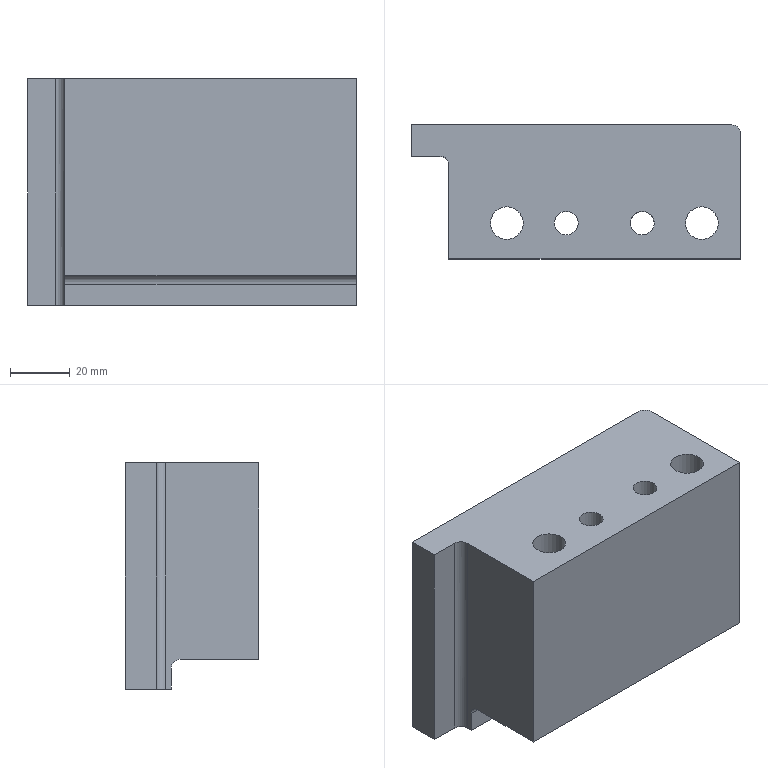Part | NX | features solid 2 | 1 solid | 25 faces | box 110.531 x 45 x 76 mm | volume 284974 mm3 | plane 14 | cylinder 11 | commonest cylinder face diameters 6 x3 8 x2 10.505 x2 11 x2 17 x2
STEP:
#1=CARTESIAN_POINT('',(699.977,-158.1,-43.001));
#2=VERTEX_POINT('',#1);
#3=CARTESIAN_POINT('',(699.977,-147.619,-43.001));
#4=VERTEX_POINT('',#3);
#5=CARTESIAN_POINT('',(699.977,-110.331,-43.001));
#6=DIRECTION('',(0.,-1.,-0.000000517));
#7=VECTOR('',#6,1000.);
#8=LINE('',#5,#7);
#9=EDGE_CURVE('',#2,#4,#8,.F.);
#10=ORIENTED_EDGE('',*,*,#9,.F.);
#11=CARTESIAN_POINT('',(699.977,-158.1,32.999));
#12=VERTEX_POINT('',#11);
#13=CARTESIAN_POINT('',(699.977,-158.101,-70.8));
#14=DIRECTION('',(0.000000053,0.000003911,1.));
#15=VECTOR('',#14,1000.);
#16=LINE('',#13,#15);
#17=EDGE_CURVE('',#12,#2,#16,.F.);
#18=ORIENTED_EDGE('',*,*,#17,.F.);
#19=CARTESIAN_POINT('',(699.977,-147.619,32.999));
#20=VERTEX_POINT('',#19);
#21=CARTESIAN_POINT('',(699.977,-187.619,32.999));
#22=DIRECTION('',(0.,1.,0.000000517));
#23=VECTOR('',#22,1000.);
#24=LINE('',#21,#23);
#25=EDGE_CURVE('',#20,#12,#24,.F.);
#26=ORIENTED_EDGE('',*,*,#25,.F.);
#27=CARTESIAN_POINT('',(699.977,-147.619,56.368));
#28=DIRECTION('',(0.000000053,-0.000000517,1.));
#29=VECTOR('',#28,1000.);
#30=LINE('',#27,#29);
#31=EDGE_CURVE('',#20,#4,#30,.F.);
#32=ORIENTED_EDGE('',*,*,#31,.T.);
#33=EDGE_LOOP('',(#10,#18,#26,#32));
#34=FACE_BOUND('',#33,.T.);
#35=CARTESIAN_POINT('',(699.977,-147.619,-43.001));
#36=DIRECTION('',(1.,0.,-0.000000053));
#37=DIRECTION('',(0.000000053,0.,1.));
#38=AXIS2_PLACEMENT_3D('',#35,#36,#37);
#39=PLANE('',#38);
#40=ADVANCED_FACE('',(#34),#39,.F.);
#41=CARTESIAN_POINT('',(807.509,-147.619,-43.001));
#42=VERTEX_POINT('',#41);
#43=CARTESIAN_POINT('',(574.977,-147.619,-43.001));
#44=DIRECTION('',(1.,0.,-0.000000053));
#45=VECTOR('',#44,1000.);
#46=LINE('',#43,#45);
#47=EDGE_CURVE('',#4,#42,#46,.T.);
#48=ORIENTED_EDGE('',*,*,#47,.T.);
#49=CARTESIAN_POINT('',(810.509,-150.619,-43.001));
#50=VERTEX_POINT('',#49);
#51=CARTESIAN_POINT('',(807.509,-150.619,-43.001));
#52=DIRECTION('',(-0.000000053,0.000000517,-1.));
#53=DIRECTION('',(0.,-1.,-0.000000517));
#54=AXIS2_PLACEMENT_3D('',#51,#52,#53);
#55=CIRCLE('',#54,3.);
#56=EDGE_CURVE('',#50,#42,#55,.F.);
#57=ORIENTED_EDGE('',*,*,#56,.F.);
#58=CARTESIAN_POINT('',(810.509,-163.1,-43.001));
#59=VERTEX_POINT('',#58);
#60=CARTESIAN_POINT('',(810.509,-177.619,-43.001));
#61=DIRECTION('',(0.,1.,0.000000517));
#62=VECTOR('',#61,1000.);
#63=LINE('',#60,#62);
#64=EDGE_CURVE('',#59,#50,#63,.T.);
#65=ORIENTED_EDGE('',*,*,#64,.F.);
#66=CARTESIAN_POINT('',(712.498,-163.1,-43.001));
#67=VERTEX_POINT('',#66);
#68=CARTESIAN_POINT('',(574.977,-163.1,-43.001));
#69=DIRECTION('',(-1.,0.,0.000000053));
#70=VECTOR('',#69,1000.);
#71=LINE('',#68,#70);
#72=EDGE_CURVE('',#59,#67,#71,.T.);
#73=ORIENTED_EDGE('',*,*,#72,.T.);
#74=CARTESIAN_POINT('',(712.498,-161.1,-43.001));
#75=VERTEX_POINT('',#74);
#76=CARTESIAN_POINT('',(712.498,-110.331,-43.001));
#77=DIRECTION('',(0.,1.,0.000000517));
#78=VECTOR('',#77,1000.);
#79=LINE('',#76,#78);
#80=EDGE_CURVE('',#67,#75,#79,.T.);
#81=ORIENTED_EDGE('',*,*,#80,.T.);
#82=CARTESIAN_POINT('',(709.498,-158.1,-43.001));
#83=VERTEX_POINT('',#82);
#84=CARTESIAN_POINT('',(709.498,-161.1,-43.001));
#85=DIRECTION('',(-0.000000053,0.000000517,-1.));
#86=DIRECTION('',(-0.01202,0.9999,0.000000518));
#87=AXIS2_PLACEMENT_3D('',#84,#85,#86);
#88=ELLIPSE('',#87,3.,3.);
#89=EDGE_CURVE('',#75,#83,#88,.F.);
#90=ORIENTED_EDGE('',*,*,#89,.T.);
#91=CARTESIAN_POINT('',(574.977,-158.1,-43.001));
#92=DIRECTION('',(1.,0.,-0.000000053));
#93=VECTOR('',#92,1000.);
#94=LINE('',#91,#93);
#95=EDGE_CURVE('',#83,#2,#94,.F.);
#96=ORIENTED_EDGE('',*,*,#95,.T.);
#97=ORIENTED_EDGE('',*,*,#9,.T.);
#98=EDGE_LOOP('',(#48,#57,#65,#73,#81,#90,#96,#97));
#99=FACE_BOUND('',#98,.T.);
#100=CARTESIAN_POINT('',(574.977,-110.331,-43.001));
#101=DIRECTION('',(-0.000000053,0.000000517,-1.));
#102=DIRECTION('',(1.,0.,-0.000000053));
#103=AXIS2_PLACEMENT_3D('',#100,#101,#102);
#104=PLANE('',#103);
#105=ADVANCED_FACE('',(#99),#104,.T.);
#106=CARTESIAN_POINT('',(807.509,-147.619,32.999));
#107=VERTEX_POINT('',#106);
#108=CARTESIAN_POINT('',(699.977,-147.619,32.999));
#109=DIRECTION('',(-1.,0.,0.000000053));
#110=VECTOR('',#109,1000.);
#111=LINE('',#108,#110);
#112=EDGE_CURVE('',#20,#107,#111,.F.);
#113=ORIENTED_EDGE('',*,*,#112,.T.);
#114=CARTESIAN_POINT('',(807.509,-147.619,56.368));
#115=DIRECTION('',(-0.000000053,0.000000517,-1.));
#116=VECTOR('',#115,1000.);
#117=LINE('',#114,#116);
#118=EDGE_CURVE('',#42,#107,#117,.F.);
#119=ORIENTED_EDGE('',*,*,#118,.F.);
#120=ORIENTED_EDGE('',*,*,#47,.F.);
#121=ORIENTED_EDGE('',*,*,#31,.F.);
#122=EDGE_LOOP('',(#113,#119,#120,#121));
#123=FACE_BOUND('',#122,.T.);
#124=CARTESIAN_POINT('',(583.446,-147.619,56.368));
#125=DIRECTION('',(0.,-1.,-0.000000517));
#126=DIRECTION('',(-0.000000053,0.000000517,-1.));
#127=AXIS2_PLACEMENT_3D('',#124,#125,#126);
#128=PLANE('',#127);
#129=ADVANCED_FACE('',(#123),#128,.F.);
#130=ORIENTED_EDGE('',*,*,#95,.F.);
#131=CARTESIAN_POINT('',(709.498,-158.1,32.999));
#132=VERTEX_POINT('',#131);
#133=CARTESIAN_POINT('',(709.498,-158.1,32.999));
#134=DIRECTION('',(0.,-0.000003911,-1.));
#135=VECTOR('',#134,1000.);
#136=LINE('',#133,#135);
#137=EDGE_CURVE('',#83,#132,#136,.F.);
#138=ORIENTED_EDGE('',*,*,#137,.T.);
#139=CARTESIAN_POINT('',(699.977,-158.1,32.999));
#140=DIRECTION('',(-1.,0.,0.000000053));
#141=VECTOR('',#140,1000.);
#142=LINE('',#139,#141);
#143=EDGE_CURVE('',#132,#12,#142,.T.);
#144=ORIENTED_EDGE('',*,*,#143,.T.);
#145=ORIENTED_EDGE('',*,*,#17,.T.);
#146=EDGE_LOOP('',(#130,#138,#144,#145));
#147=FACE_BOUND('',#146,.T.);
#148=CARTESIAN_POINT('',(704.737,-158.1,-5.001));
#149=DIRECTION('',(0.,-1.,0.000003911));
#150=DIRECTION('',(0.,-0.000003911,-1.));
#151=AXIS2_PLACEMENT_3D('',#148,#149,#150);
#152=PLANE('',#151);
#153=ADVANCED_FACE('',(#147),#152,.T.);
#154=ORIENTED_EDGE('',*,*,#143,.F.);
#155=CARTESIAN_POINT('',(712.498,-161.1,32.999));
#156=VERTEX_POINT('',#155);
#157=CARTESIAN_POINT('',(709.498,-161.1,32.999));
#158=DIRECTION('',(0.000000053,-0.000000517,1.));
#159=DIRECTION('',(-0.01202,0.9999,0.000000518));
#160=AXIS2_PLACEMENT_3D('',#157,#158,#159);
#161=ELLIPSE('',#160,3.,3.);
#162=EDGE_CURVE('',#132,#156,#161,.F.);
#163=ORIENTED_EDGE('',*,*,#162,.T.);
#164=CARTESIAN_POINT('',(712.498,-192.619,32.999));
#165=VERTEX_POINT('',#164);
#166=CARTESIAN_POINT('',(712.498,-187.619,32.999));
#167=DIRECTION('',(0.,-1.,-0.000000517));
#168=VECTOR('',#167,1000.);
#169=LINE('',#166,#168);
#170=EDGE_CURVE('',#165,#156,#169,.F.);
#171=ORIENTED_EDGE('',*,*,#170,.F.);
#172=CARTESIAN_POINT('',(810.509,-192.619,32.999));
#173=VERTEX_POINT('',#172);
#174=CARTESIAN_POINT('',(699.977,-192.619,32.999));
#175=DIRECTION('',(-1.,0.,0.000000053));
#176=VECTOR('',#175,1000.);
#177=LINE('',#174,#176);
#178=EDGE_CURVE('',#165,#173,#177,.F.);
#179=ORIENTED_EDGE('',*,*,#178,.T.);
#180=CARTESIAN_POINT('',(810.509,-150.619,32.999));
#181=VERTEX_POINT('',#180);
#182=CARTESIAN_POINT('',(810.509,-177.619,32.999));
#183=DIRECTION('',(0.,-1.,-0.000000517));
#184=VECTOR('',#183,1000.);
#185=LINE('',#182,#184);
#186=EDGE_CURVE('',#173,#181,#185,.F.);
#187=ORIENTED_EDGE('',*,*,#186,.T.);
#188=CARTESIAN_POINT('',(807.509,-150.619,32.999));
#189=DIRECTION('',(0.000000053,-0.000000517,1.));
#190=DIRECTION('',(0.,1.,0.000000517));
#191=AXIS2_PLACEMENT_3D('',#188,#189,#190);
#192=CIRCLE('',#191,3.);
#193=EDGE_CURVE('',#181,#107,#192,.T.);
#194=ORIENTED_EDGE('',*,*,#193,.T.);
#195=ORIENTED_EDGE('',*,*,#112,.F.);
#196=ORIENTED_EDGE('',*,*,#25,.T.);
#197=EDGE_LOOP('',(#154,#163,#171,#179,#187,#194,#195,#196));
#198=FACE_BOUND('',#197,.T.);
#199=CARTESIAN_POINT('',(797.509,-186.119,32.999));
#200=VERTEX_POINT('',#199);
#201=CARTESIAN_POINT('',(797.509,-180.619,32.999));
#202=DIRECTION('',(0.000000053,-0.000000517,1.));
#203=DIRECTION('',(0.,-1.,-0.000000517));
#204=AXIS2_PLACEMENT_3D('',#201,#202,#203);
#205=CIRCLE('',#204,5.5);
#206=EDGE_CURVE('',#200,#200,#205,.F.);
#207=ORIENTED_EDGE('',*,*,#206,.T.);
#208=EDGE_LOOP('',(#207));
#209=FACE_BOUND('',#208,.T.);
#210=CARTESIAN_POINT('',(731.977,-186.119,32.999));
#211=VERTEX_POINT('',#210);
#212=CARTESIAN_POINT('',(731.977,-180.619,32.999));
#213=DIRECTION('',(0.000000053,-0.000000517,1.));
#214=DIRECTION('',(0.,-1.,-0.000000517));
#215=AXIS2_PLACEMENT_3D('',#212,#213,#214);
#216=CIRCLE('',#215,5.5);
#217=EDGE_CURVE('',#211,#211,#216,.F.);
#218=ORIENTED_EDGE('',*,*,#217,.T.);
#219=EDGE_LOOP('',(#218));
#220=FACE_BOUND('',#219,.T.);
#221=CARTESIAN_POINT('',(777.509,-184.619,32.999));
#222=VERTEX_POINT('',#221);
#223=CARTESIAN_POINT('',(777.509,-180.619,32.999));
#224=DIRECTION('',(-0.000000053,0.000000517,-1.));
#225=DIRECTION('',(0.,-1.,-0.000000517));
#226=AXIS2_PLACEMENT_3D('',#223,#224,#225);
#227=CIRCLE('',#226,4.);
#228=EDGE_CURVE('',#222,#222,#227,.T.);
#229=ORIENTED_EDGE('',*,*,#228,.T.);
#230=EDGE_LOOP('',(#229));
#231=FACE_BOUND('',#230,.T.);
#232=CARTESIAN_POINT('',(751.977,-184.619,32.999));
#233=VERTEX_POINT('',#232);
#234=CARTESIAN_POINT('',(751.977,-180.619,32.999));
#235=DIRECTION('',(-0.000000053,0.000000517,-1.));
#236=DIRECTION('',(0.,-1.,-0.000000517));
#237=AXIS2_PLACEMENT_3D('',#234,#235,#236);
#238=CIRCLE('',#237,4.);
#239=EDGE_CURVE('',#233,#233,#238,.T.);
#240=ORIENTED_EDGE('',*,*,#239,.T.);
#241=EDGE_LOOP('',(#240));
#242=FACE_BOUND('',#241,.T.);
#243=CARTESIAN_POINT('',(699.977,-187.619,32.999));
#244=DIRECTION('',(0.000000053,-0.000000517,1.));
#245=DIRECTION('',(1.,0.,-0.000000053));
#246=AXIS2_PLACEMENT_3D('',#243,#244,#245);
#247=PLANE('',#246);
#248=ADVANCED_FACE('',(#198,#209,#220,#231,#242),#247,.T.);
#249=CARTESIAN_POINT('',(810.509,-163.1,-36.001));
#250=VERTEX_POINT('',#249);
#251=CARTESIAN_POINT('',(810.509,-163.1,-5.001));
#252=DIRECTION('',(0.000000053,0.000003911,1.));
#253=VECTOR('',#252,1000.);
#254=LINE('',#251,#253);
#255=EDGE_CURVE('',#59,#250,#254,.T.);
#256=ORIENTED_EDGE('',*,*,#255,.T.);
#257=CARTESIAN_POINT('',(712.498,-163.1,-36.001));
#258=VERTEX_POINT('',#257);
#259=CARTESIAN_POINT('',(712.498,-163.1,-36.001));
#260=DIRECTION('',(1.,0.,-0.000000053));
#261=VECTOR('',#260,1000.);
#262=LINE('',#259,#261);
#263=EDGE_CURVE('',#250,#258,#262,.F.);
#264=ORIENTED_EDGE('',*,*,#263,.T.);
#265=CARTESIAN_POINT('',(712.498,-163.1,49.2));
#266=DIRECTION('',(0.,0.000003911,1.));
#267=VECTOR('',#266,1000.);
#268=LINE('',#265,#267);
#269=EDGE_CURVE('',#67,#258,#268,.T.);
#270=ORIENTED_EDGE('',*,*,#269,.F.);
#271=ORIENTED_EDGE('',*,*,#72,.F.);
#272=EDGE_LOOP('',(#256,#264,#270,#271));
#273=FACE_BOUND('',#272,.T.);
#274=CARTESIAN_POINT('',(704.737,-163.1,-5.001));
#275=DIRECTION('',(0.,-1.,0.000003911));
#276=DIRECTION('',(0.,-0.000003911,-1.));
#277=AXIS2_PLACEMENT_3D('',#274,#275,#276);
#278=PLANE('',#277);
#279=ADVANCED_FACE('',(#273),#278,.T.);
#280=ORIENTED_EDGE('',*,*,#186,.F.);
#281=CARTESIAN_POINT('',(810.509,-192.619,-33.001));
#282=VERTEX_POINT('',#281);
#283=CARTESIAN_POINT('',(810.509,-192.619,-43.001));
#284=DIRECTION('',(0.000000053,-0.000000517,1.));
#285=VECTOR('',#284,1000.);
#286=LINE('',#283,#285);
#287=EDGE_CURVE('',#173,#282,#286,.F.);
#288=ORIENTED_EDGE('',*,*,#287,.T.);
#289=CARTESIAN_POINT('',(810.509,-166.1,-33.001));
#290=VERTEX_POINT('',#289);
#291=CARTESIAN_POINT('',(810.509,-177.619,-33.001));
#292=DIRECTION('',(0.,1.,0.000000517));
#293=VECTOR('',#292,1000.);
#294=LINE('',#291,#293);
#295=EDGE_CURVE('',#282,#290,#294,.T.);
#296=ORIENTED_EDGE('',*,*,#295,.T.);
#297=CARTESIAN_POINT('',(810.509,-166.1,-36.001));
#298=DIRECTION('',(1.,0.,-0.000000053));
#299=DIRECTION('',(-0.000000053,0.,-1.));
#300=AXIS2_PLACEMENT_3D('',#297,#298,#299);
#301=CIRCLE('',#300,3.);
#302=EDGE_CURVE('',#290,#250,#301,.F.);
#303=ORIENTED_EDGE('',*,*,#302,.T.);
#304=ORIENTED_EDGE('',*,*,#255,.F.);
#305=ORIENTED_EDGE('',*,*,#64,.T.);
#306=CARTESIAN_POINT('',(810.509,-150.619,-43.001));
#307=DIRECTION('',(-0.000000053,0.000000517,-1.));
#308=VECTOR('',#307,1000.);
#309=LINE('',#306,#308);
#310=EDGE_CURVE('',#181,#50,#309,.T.);
#311=ORIENTED_EDGE('',*,*,#310,.F.);
#312=EDGE_LOOP('',(#280,#288,#296,#303,#304,#305,#311));
#313=FACE_BOUND('',#312,.T.);
#314=CARTESIAN_POINT('',(810.509,-177.619,-43.001));
#315=DIRECTION('',(1.,0.,-0.000000053));
#316=DIRECTION('',(0.000000053,-0.000000517,1.));
#317=AXIS2_PLACEMENT_3D('',#314,#315,#316);
#318=PLANE('',#317);
#319=ADVANCED_FACE('',(#313),#318,.T.);
#320=ORIENTED_EDGE('',*,*,#178,.F.);
#321=CARTESIAN_POINT('',(712.498,-192.619,-33.001));
#322=VERTEX_POINT('',#321);
#323=CARTESIAN_POINT('',(712.498,-192.619,-43.001));
#324=DIRECTION('',(0.,0.000000517,-1.));
#325=VECTOR('',#324,1000.);
#326=LINE('',#323,#325);
#327=EDGE_CURVE('',#165,#322,#326,.T.);
#328=ORIENTED_EDGE('',*,*,#327,.T.);
#329=CARTESIAN_POINT('',(574.977,-192.619,-33.001));
#330=DIRECTION('',(-1.,0.,0.000000053));
#331=VECTOR('',#330,1000.);
#332=LINE('',#329,#331);
#333=EDGE_CURVE('',#282,#322,#332,.T.);
#334=ORIENTED_EDGE('',*,*,#333,.F.);
#335=ORIENTED_EDGE('',*,*,#287,.F.);
#336=EDGE_LOOP('',(#320,#328,#334,#335));
#337=FACE_BOUND('',#336,.T.);
#338=CARTESIAN_POINT('',(699.977,-192.619,-43.001));
#339=DIRECTION('',(0.,-1.,-0.000000517));
#340=DIRECTION('',(-0.000000053,0.000000517,-1.));
#341=AXIS2_PLACEMENT_3D('',#338,#339,#340);
#342=PLANE('',#341);
#343=ADVANCED_FACE('',(#337),#342,.T.);
#344=ORIENTED_EDGE('',*,*,#170,.T.);
#345=CARTESIAN_POINT('',(712.498,-161.1,-43.001));
#346=DIRECTION('',(0.,-0.000003911,-1.));
#347=VECTOR('',#346,1000.);
#348=LINE('',#345,#347);
#349=EDGE_CURVE('',#156,#75,#348,.T.);
#350=ORIENTED_EDGE('',*,*,#349,.T.);
#351=ORIENTED_EDGE('',*,*,#80,.F.);
#352=ORIENTED_EDGE('',*,*,#269,.T.);
#353=CARTESIAN_POINT('',(712.498,-166.1,-33.001));
#354=VERTEX_POINT('',#353);
#355=CARTESIAN_POINT('',(712.498,-166.1,-36.001));
#356=DIRECTION('',(-1.,0.,0.));
#357=DIRECTION('',(0.,-1.,0.));
#358=AXIS2_PLACEMENT_3D('',#355,#356,#357);
#359=CIRCLE('',#358,3.);
#360=EDGE_CURVE('',#258,#354,#359,.F.);
#361=ORIENTED_EDGE('',*,*,#360,.T.);
#362=CARTESIAN_POINT('',(712.498,-110.331,-33.001));
#363=DIRECTION('',(0.,1.,0.000000517));
#364=VECTOR('',#363,1000.);
#365=LINE('',#362,#364);
#366=EDGE_CURVE('',#322,#354,#365,.T.);
#367=ORIENTED_EDGE('',*,*,#366,.F.);
#368=ORIENTED_EDGE('',*,*,#327,.F.);
#369=EDGE_LOOP('',(#344,#350,#351,#352,#361,#367,#368));
#370=FACE_BOUND('',#369,.T.);
#371=CARTESIAN_POINT('',(712.498,-177.1,49.2));
#372=DIRECTION('',(-1.,0.,0.));
#373=DIRECTION('',(0.,-1.,0.000003329));
#374=AXIS2_PLACEMENT_3D('',#371,#372,#373);
#375=PLANE('',#374);
#376=ADVANCED_FACE('',(#370),#375,.T.);
#377=ORIENTED_EDGE('',*,*,#366,.T.);
#378=CARTESIAN_POINT('',(810.509,-166.1,-33.001));
#379=DIRECTION('',(1.,0.,-0.000000053));
#380=VECTOR('',#379,1000.);
#381=LINE('',#378,#380);
#382=EDGE_CURVE('',#354,#290,#381,.T.);
#383=ORIENTED_EDGE('',*,*,#382,.T.);
#384=ORIENTED_EDGE('',*,*,#295,.F.);
#385=ORIENTED_EDGE('',*,*,#333,.T.);
#386=EDGE_LOOP('',(#377,#383,#384,#385));
#387=FACE_BOUND('',#386,.T.);
#388=CARTESIAN_POINT('',(731.977,-172.119,-33.001));
#389=VERTEX_POINT('',#388);
#390=CARTESIAN_POINT('',(731.977,-180.619,-33.001));
#391=DIRECTION('',(-0.000000053,0.000000517,-1.));
#392=DIRECTION('',(0.,1.,0.000000517));
#393=AXIS2_PLACEMENT_3D('',#390,#391,#392);
#394=CIRCLE('',#393,8.5);
#395=EDGE_CURVE('',#389,#389,#394,.T.);
#396=ORIENTED_EDGE('',*,*,#395,.F.);
#397=EDGE_LOOP('',(#396));
#398=FACE_BOUND('',#397,.T.);
#399=CARTESIAN_POINT('',(751.977,-175.366,-33.001));
#400=VERTEX_POINT('',#399);
#401=CARTESIAN_POINT('',(753.045,-175.439,-33.001));
#402=CARTESIAN_POINT('',(752.012,-175.332,-33.001));
#403=CARTESIAN_POINT('',(750.981,-175.429,-33.001));
#404=CARTESIAN_POINT('',(750.004,-175.714,-33.001));
#405=CARTESIAN_POINT('',(749.086,-176.193,-33.001));
#406=CARTESIAN_POINT('',(748.278,-176.842,-33.001));
#407=CARTESIAN_POINT('',(747.613,-177.636,-33.001));
#408=CARTESIAN_POINT('',(747.115,-178.545,-33.001));
#409=CARTESIAN_POINT('',(746.803,-179.533,-33.001));
#410=CARTESIAN_POINT('',(746.691,-180.564,-33.001));
#411=CARTESIAN_POINT('',(746.782,-181.596,-33.001));
#412=CARTESIAN_POINT('',(747.073,-182.591,-33.001));
#413=CARTESIAN_POINT('',(747.552,-183.51,-33.001));
#414=CARTESIAN_POINT('',(748.201,-184.318,-33.001));
#415=CARTESIAN_POINT('',(748.995,-184.983,-33.001));
#416=CARTESIAN_POINT('',(749.904,-185.481,-33.001));
#417=CARTESIAN_POINT('',(750.892,-185.792,-33.001));
#418=CARTESIAN_POINT('',(751.922,-185.905,-33.001));
#419=CARTESIAN_POINT('',(752.955,-185.814,-33.001));
#420=CARTESIAN_POINT('',(753.95,-185.523,-33.001));
#421=CARTESIAN_POINT('',(754.868,-185.044,-33.001));
#422=CARTESIAN_POINT('',(755.676,-184.395,-33.001));
#423=CARTESIAN_POINT('',(756.342,-183.601,-33.001));
#424=CARTESIAN_POINT('',(756.84,-182.692,-33.001));
#425=CARTESIAN_POINT('',(757.151,-181.704,-33.001));
#426=CARTESIAN_POINT('',(757.263,-180.673,-33.001));
#427=CARTESIAN_POINT('',(757.172,-179.641,-33.001));
#428=CARTESIAN_POINT('',(756.882,-178.646,-33.001));
#429=CARTESIAN_POINT('',(756.403,-177.727,-33.001));
#430=CARTESIAN_POINT('',(755.754,-176.919,-33.001));
#431=CARTESIAN_POINT('',(754.96,-176.254,-33.001));
#432=CARTESIAN_POINT('',(754.051,-175.756,-33.001));
#433=CARTESIAN_POINT('',(753.045,-175.439,-33.001));
#434=CARTESIAN_POINT('',(752.012,-175.332,-33.001));
#435=CARTESIAN_POINT('',(750.981,-175.429,-33.001));
#436=B_SPLINE_CURVE_WITH_KNOTS('',3,(#401,#402,#403,#404,#405,#406,#407,#408,#409,#410,#411,#412,#413,#414,#415,#416,#417,#418,#419,#420,#421,#422,#423,#424,#425,#426,#427,#428,#429,#430,#431,#432,#433,#434,#435),.UNSPECIFIED.,.T.,.F.,(1,1,1,1,1,1,1,1,1,1,1,1,1,1,1,1,1,1,1,1,1,1,1,1,1,1,1,1,1,1,1,1,1,1,1,1,1,1,1),(-0.09539,-0.06414,-0.03289,0.,0.02969,0.06086,0.09211,0.1234,0.1546,0.1859,0.2171,0.2484,0.2796,0.3109,0.3421,0.3734,0.4046,0.4359,0.4671,0.4984,0.5296,0.5609,0.5921,0.6234,0.6546,0.6859,0.7171,0.7484,0.7796,0.8109,0.8421,0.8734,0.9046,0.9359,0.9671,1.,1.03,1.061,1.092),.UNSPECIFIED.);
#437=EDGE_CURVE('',#400,#400,#436,.F.);
#438=ORIENTED_EDGE('',*,*,#437,.F.);
#439=EDGE_LOOP('',(#438));
#440=FACE_BOUND('',#439,.T.);
#441=CARTESIAN_POINT('',(777.509,-175.366,-33.001));
#442=VERTEX_POINT('',#441);
#443=CARTESIAN_POINT('',(776.441,-175.439,-33.001));
#444=CARTESIAN_POINT('',(777.473,-175.332,-33.001));
#445=CARTESIAN_POINT('',(778.504,-175.429,-33.001));
#446=CARTESIAN_POINT('',(779.482,-175.714,-33.001));
#447=CARTESIAN_POINT('',(780.4,-176.193,-33.001));
#448=CARTESIAN_POINT('',(781.208,-176.842,-33.001));
#449=CARTESIAN_POINT('',(781.873,-177.636,-33.001));
#450=CARTESIAN_POINT('',(782.371,-178.545,-33.001));
#451=CARTESIAN_POINT('',(782.682,-179.533,-33.001));
#452=CARTESIAN_POINT('',(782.795,-180.564,-33.001));
#453=CARTESIAN_POINT('',(782.704,-181.596,-33.001));
#454=CARTESIAN_POINT('',(782.413,-182.591,-33.001));
#455=CARTESIAN_POINT('',(781.934,-183.51,-33.001));
#456=CARTESIAN_POINT('',(781.285,-184.318,-33.001));
#457=CARTESIAN_POINT('',(780.491,-184.983,-33.001));
#458=CARTESIAN_POINT('',(779.582,-185.481,-33.001));
#459=CARTESIAN_POINT('',(778.594,-185.792,-33.001));
#460=CARTESIAN_POINT('',(777.563,-185.905,-33.001));
#461=CARTESIAN_POINT('',(776.531,-185.814,-33.001));
#462=CARTESIAN_POINT('',(775.536,-185.523,-33.001));
#463=CARTESIAN_POINT('',(774.617,-185.044,-33.001));
#464=CARTESIAN_POINT('',(773.81,-184.395,-33.001));
#465=CARTESIAN_POINT('',(773.144,-183.601,-33.001));
#466=CARTESIAN_POINT('',(772.646,-182.692,-33.001));
#467=CARTESIAN_POINT('',(772.335,-181.704,-33.001));
#468=CARTESIAN_POINT('',(772.222,-180.673,-33.001));
#469=CARTESIAN_POINT('',(772.313,-179.641,-33.001));
#470=CARTESIAN_POINT('',(772.604,-178.646,-33.001));
#471=CARTESIAN_POINT('',(773.083,-177.727,-33.001));
#472=CARTESIAN_POINT('',(773.732,-176.919,-33.001));
#473=CARTESIAN_POINT('',(774.526,-176.254,-33.001));
#474=CARTESIAN_POINT('',(775.435,-175.756,-33.001));
#475=CARTESIAN_POINT('',(776.441,-175.439,-33.001));
#476=CARTESIAN_POINT('',(777.473,-175.332,-33.001));
#477=CARTESIAN_POINT('',(778.504,-175.429,-33.001));
#478=B_SPLINE_CURVE_WITH_KNOTS('',3,(#443,#444,#445,#446,#447,#448,#449,#450,#451,#452,#453,#454,#455,#456,#457,#458,#459,#460,#461,#462,#463,#464,#465,#466,#467,#468,#469,#470,#471,#472,#473,#474,#475,#476,#477),.UNSPECIFIED.,.T.,.F.,(1,1,1,1,1,1,1,1,1,1,1,1,1,1,1,1,1,1,1,1,1,1,1,1,1,1,1,1,1,1,1,1,1,1,1,1,1,1,1),(-0.09539,-0.06414,-0.03289,0.,0.02969,0.06086,0.09211,0.1234,0.1546,0.1859,0.2171,0.2484,0.2796,0.3109,0.3421,0.3734,0.4046,0.4359,0.4671,0.4984,0.5296,0.5609,0.5921,0.6234,0.6546,0.6859,0.7171,0.7484,0.7796,0.8109,0.8421,0.8734,0.9046,0.9359,0.9671,1.,1.03,1.061,1.092),.UNSPECIFIED.);
#479=EDGE_CURVE('',#442,#442,#478,.T.);
#480=ORIENTED_EDGE('',*,*,#479,.F.);
#481=EDGE_LOOP('',(#480));
#482=FACE_BOUND('',#481,.T.);
#483=CARTESIAN_POINT('',(797.509,-172.119,-33.001));
#484=VERTEX_POINT('',#483);
#485=CARTESIAN_POINT('',(797.509,-180.619,-33.001));
#486=DIRECTION('',(-0.000000053,0.000000517,-1.));
#487=DIRECTION('',(0.,1.,0.000000517));
#488=AXIS2_PLACEMENT_3D('',#485,#486,#487);
#489=CIRCLE('',#488,8.5);
#490=EDGE_CURVE('',#484,#484,#489,.T.);
#491=ORIENTED_EDGE('',*,*,#490,.F.);
#492=EDGE_LOOP('',(#491));
#493=FACE_BOUND('',#492,.T.);
#494=CARTESIAN_POINT('',(574.977,-110.331,-33.001));
#495=DIRECTION('',(-0.000000053,0.000000517,-1.));
#496=DIRECTION('',(1.,0.,-0.000000053));
#497=AXIS2_PLACEMENT_3D('',#494,#495,#496);
#498=PLANE('',#497);
#499=ADVANCED_FACE('',(#387,#398,#440,#482,#493),#498,.T.);
#500=CARTESIAN_POINT('',(797.509,-175.119,7.999));
#501=VERTEX_POINT('',#500);
#502=CARTESIAN_POINT('',(797.509,-180.619,7.999));
#503=DIRECTION('',(-0.00000016,0.000000517,-1.));
#504=DIRECTION('',(0.,1.,0.000000517));
#505=AXIS2_PLACEMENT_3D('',#502,#503,#504);
#506=CIRCLE('',#505,5.5);
#507=EDGE_CURVE('',#501,#501,#506,.T.);
#508=ORIENTED_EDGE('',*,*,#507,.T.);
#509=EDGE_LOOP('',(#508));
#510=FACE_BOUND('',#509,.T.);
#511=ORIENTED_EDGE('',*,*,#206,.F.);
#512=EDGE_LOOP('',(#511));
#513=FACE_BOUND('',#512,.T.);
#514=CARTESIAN_POINT('',(797.509,-180.619,33.999));
#515=DIRECTION('',(-0.00000016,0.000000517,-1.));
#516=DIRECTION('',(0.,-1.,-0.000000517));
#517=AXIS2_PLACEMENT_3D('',#514,#515,#516);
#518=CYLINDRICAL_SURFACE('',#517,5.5);
#519=ADVANCED_FACE('',(#510,#513),#518,.F.);
#520=ORIENTED_EDGE('',*,*,#490,.T.);
#521=EDGE_LOOP('',(#520));
#522=FACE_BOUND('',#521,.T.);
#523=CARTESIAN_POINT('',(797.509,-172.119,7.999));
#524=VERTEX_POINT('',#523);
#525=CARTESIAN_POINT('',(797.509,-180.619,7.999));
#526=DIRECTION('',(-0.00000016,0.000000517,-1.));
#527=DIRECTION('',(0.,1.,0.000000517));
#528=AXIS2_PLACEMENT_3D('',#525,#526,#527);
#529=CIRCLE('',#528,8.5);
#530=EDGE_CURVE('',#524,#524,#529,.F.);
#531=ORIENTED_EDGE('',*,*,#530,.T.);
#532=EDGE_LOOP('',(#531));
#533=FACE_BOUND('',#532,.T.);
#534=CARTESIAN_POINT('',(797.509,-180.619,7.999));
#535=DIRECTION('',(-0.00000016,0.000000517,-1.));
#536=DIRECTION('',(0.,-1.,-0.000000517));
#537=AXIS2_PLACEMENT_3D('',#534,#535,#536);
#538=CYLINDRICAL_SURFACE('',#537,8.5);
#539=ADVANCED_FACE('',(#522,#533),#538,.F.);
#540=ORIENTED_EDGE('',*,*,#507,.F.);
#541=EDGE_LOOP('',(#540));
#542=FACE_BOUND('',#541,.T.);
#543=ORIENTED_EDGE('',*,*,#530,.F.);
#544=EDGE_LOOP('',(#543));
#545=FACE_BOUND('',#544,.T.);
#546=CARTESIAN_POINT('',(797.509,-180.619,7.999));
#547=DIRECTION('',(-0.00000016,0.000000517,-1.));
#548=DIRECTION('',(0.,-1.,-0.000000517));
#549=AXIS2_PLACEMENT_3D('',#546,#547,#548);
#550=PLANE('',#549);
#551=ADVANCED_FACE('',(#542,#545),#550,.T.);
#552=CARTESIAN_POINT('',(781.509,-180.618,-13.001));
#553=VERTEX_POINT('',#552);
#554=CARTESIAN_POINT('',(777.509,-180.618,-13.001));
#555=DIRECTION('',(-0.000000874,-0.000001551,1.));
#556=DIRECTION('',(1.,0.,0.000000874));
#557=AXIS2_PLACEMENT_3D('',#554,#555,#556);
#558=CIRCLE('',#557,4.);
#559=EDGE_CURVE('',#553,#553,#558,.F.);
#560=ORIENTED_EDGE('',*,*,#559,.T.);
#561=EDGE_LOOP('',(#560));
#562=FACE_BOUND('',#561,.T.);
#563=ORIENTED_EDGE('',*,*,#228,.F.);
#564=EDGE_LOOP('',(#563));
#565=FACE_BOUND('',#564,.T.);
#566=CARTESIAN_POINT('',(777.509,-180.619,33.999));
#567=DIRECTION('',(0.000000874,0.000001551,-1.));
#568=DIRECTION('',(0.,-1.,-0.000001551));
#569=AXIS2_PLACEMENT_3D('',#566,#567,#568);
#570=CYLINDRICAL_SURFACE('',#569,4.);
#571=ADVANCED_FACE('',(#562,#565),#570,.F.);
#572=ORIENTED_EDGE('',*,*,#479,.T.);
#573=EDGE_LOOP('',(#572));
#574=FACE_BOUND('',#573,.T.);
#575=CARTESIAN_POINT('',(782.761,-180.618,-13.001));
#576=VERTEX_POINT('',#575);
#577=CARTESIAN_POINT('',(777.509,-180.618,-13.001));
#578=DIRECTION('',(-0.000000874,-0.000001551,1.));
#579=DIRECTION('',(1.,0.,0.000000874));
#580=AXIS2_PLACEMENT_3D('',#577,#578,#579);
#581=CIRCLE('',#580,5.253);
#582=EDGE_CURVE('',#576,#576,#581,.T.);
#583=ORIENTED_EDGE('',*,*,#582,.T.);
#584=EDGE_LOOP('',(#583));
#585=FACE_BOUND('',#584,.T.);
#586=CARTESIAN_POINT('',(777.509,-180.618,-33.001));
#587=DIRECTION('',(0.000000874,0.000001551,-1.));
#588=DIRECTION('',(0.,-1.,-0.000001551));
#589=AXIS2_PLACEMENT_3D('',#586,#587,#588);
#590=CYLINDRICAL_SURFACE('',#589,5.253);
#591=ADVANCED_FACE('',(#574,#585),#590,.F.);
#592=ORIENTED_EDGE('',*,*,#559,.F.);
#593=EDGE_LOOP('',(#592));
#594=FACE_BOUND('',#593,.T.);
#595=ORIENTED_EDGE('',*,*,#582,.F.);
#596=EDGE_LOOP('',(#595));
#597=FACE_BOUND('',#596,.T.);
#598=CARTESIAN_POINT('',(777.509,-180.618,-13.001));
#599=DIRECTION('',(0.000000874,0.000001551,-1.));
#600=DIRECTION('',(0.,-1.,-0.000001551));
#601=AXIS2_PLACEMENT_3D('',#598,#599,#600);
#602=PLANE('',#601);
#603=ADVANCED_FACE('',(#594,#597),#602,.T.);
#604=CARTESIAN_POINT('',(751.977,-184.619,-13.001));
#605=VERTEX_POINT('',#604);
#606=CARTESIAN_POINT('',(751.977,-180.619,-13.001));
#607=DIRECTION('',(0.000001087,-0.000001551,1.));
#608=DIRECTION('',(0.,-1.,-0.000001551));
#609=AXIS2_PLACEMENT_3D('',#606,#607,#608);
#610=CIRCLE('',#609,4.);
#611=EDGE_CURVE('',#605,#605,#610,.T.);
#612=ORIENTED_EDGE('',*,*,#611,.F.);
#613=EDGE_LOOP('',(#612));
#614=FACE_BOUND('',#613,.T.);
#615=ORIENTED_EDGE('',*,*,#239,.F.);
#616=EDGE_LOOP('',(#615));
#617=FACE_BOUND('',#616,.T.);
#618=CARTESIAN_POINT('',(751.977,-180.619,33.999));
#619=DIRECTION('',(-0.000001087,0.000001551,-1.));
#620=DIRECTION('',(0.,-1.,-0.000001551));
#621=AXIS2_PLACEMENT_3D('',#618,#619,#620);
#622=CYLINDRICAL_SURFACE('',#621,4.);
#623=ADVANCED_FACE('',(#614,#617),#622,.F.);
#624=ORIENTED_EDGE('',*,*,#437,.T.);
#625=EDGE_LOOP('',(#624));
#626=FACE_BOUND('',#625,.T.);
#627=CARTESIAN_POINT('',(746.725,-180.619,-13.001));
#628=VERTEX_POINT('',#627);
#629=CARTESIAN_POINT('',(751.977,-180.619,-13.001));
#630=DIRECTION('',(0.000001087,-0.000001551,1.));
#631=DIRECTION('',(-1.,0.,0.000001087));
#632=AXIS2_PLACEMENT_3D('',#629,#630,#631);
#633=CIRCLE('',#632,5.253);
#634=EDGE_CURVE('',#628,#628,#633,.F.);
#635=ORIENTED_EDGE('',*,*,#634,.F.);
#636=EDGE_LOOP('',(#635));
#637=FACE_BOUND('',#636,.T.);
#638=CARTESIAN_POINT('',(751.977,-180.619,-33.001));
#639=DIRECTION('',(-0.000001087,0.000001551,-1.));
#640=DIRECTION('',(0.,-1.,-0.000001551));
#641=AXIS2_PLACEMENT_3D('',#638,#639,#640);
#642=CYLINDRICAL_SURFACE('',#641,5.253);
#643=ADVANCED_FACE('',(#626,#637),#642,.F.);
#644=ORIENTED_EDGE('',*,*,#611,.T.);
#645=EDGE_LOOP('',(#644));
#646=FACE_BOUND('',#645,.T.);
#647=ORIENTED_EDGE('',*,*,#634,.T.);
#648=EDGE_LOOP('',(#647));
#649=FACE_BOUND('',#648,.T.);
#650=CARTESIAN_POINT('',(751.977,-180.619,-13.001));
#651=DIRECTION('',(-0.000001087,0.000001551,-1.));
#652=DIRECTION('',(0.,-1.,-0.000001551));
#653=AXIS2_PLACEMENT_3D('',#650,#651,#652);
#654=PLANE('',#653);
#655=ADVANCED_FACE('',(#646,#649),#654,.T.);
#656=CARTESIAN_POINT('',(731.977,-175.119,7.999));
#657=VERTEX_POINT('',#656);
#658=CARTESIAN_POINT('',(731.977,-180.619,7.999));
#659=DIRECTION('',(-0.000000053,0.000000517,-1.));
#660=DIRECTION('',(0.,1.,0.000000517));
#661=AXIS2_PLACEMENT_3D('',#658,#659,#660);
#662=CIRCLE('',#661,5.5);
#663=EDGE_CURVE('',#657,#657,#662,.F.);
#664=ORIENTED_EDGE('',*,*,#663,.F.);
#665=EDGE_LOOP('',(#664));
#666=FACE_BOUND('',#665,.T.);
#667=ORIENTED_EDGE('',*,*,#217,.F.);
#668=EDGE_LOOP('',(#667));
#669=FACE_BOUND('',#668,.T.);
#670=CARTESIAN_POINT('',(731.977,-180.619,33.999));
#671=DIRECTION('',(-0.000000053,0.000000517,-1.));
#672=DIRECTION('',(0.,-1.,-0.000000517));
#673=AXIS2_PLACEMENT_3D('',#670,#671,#672);
#674=CYLINDRICAL_SURFACE('',#673,5.5);
#675=ADVANCED_FACE('',(#666,#669),#674,.F.);
#676=ORIENTED_EDGE('',*,*,#395,.T.);
#677=EDGE_LOOP('',(#676));
#678=FACE_BOUND('',#677,.T.);
#679=CARTESIAN_POINT('',(731.977,-172.119,7.999));
#680=VERTEX_POINT('',#679);
#681=CARTESIAN_POINT('',(731.977,-180.619,7.999));
#682=DIRECTION('',(-0.000000053,0.000000517,-1.));
#683=DIRECTION('',(0.,1.,0.000000517));
#684=AXIS2_PLACEMENT_3D('',#681,#682,#683);
#685=CIRCLE('',#684,8.5);
#686=EDGE_CURVE('',#680,#680,#685,.T.);
#687=ORIENTED_EDGE('',*,*,#686,.F.);
#688=EDGE_LOOP('',(#687));
#689=FACE_BOUND('',#688,.T.);
#690=CARTESIAN_POINT('',(731.977,-180.619,7.999));
#691=DIRECTION('',(-0.000000053,0.000000517,-1.));
#692=DIRECTION('',(0.,-1.,-0.000000517));
#693=AXIS2_PLACEMENT_3D('',#690,#691,#692);
#694=CYLINDRICAL_SURFACE('',#693,8.5);
#695=ADVANCED_FACE('',(#678,#689),#694,.F.);
#696=ORIENTED_EDGE('',*,*,#663,.T.);
#697=EDGE_LOOP('',(#696));
#698=FACE_BOUND('',#697,.T.);
#699=ORIENTED_EDGE('',*,*,#686,.T.);
#700=EDGE_LOOP('',(#699));
#701=FACE_BOUND('',#700,.T.);
#702=CARTESIAN_POINT('',(731.977,-180.619,7.999));
#703=DIRECTION('',(-0.000000053,0.000000517,-1.));
#704=DIRECTION('',(0.,-1.,-0.000000517));
#705=AXIS2_PLACEMENT_3D('',#702,#703,#704);
#706=PLANE('',#705);
#707=ADVANCED_FACE('',(#698,#701),#706,.T.);
#708=ORIENTED_EDGE('',*,*,#193,.F.);
#709=ORIENTED_EDGE('',*,*,#310,.T.);
#710=ORIENTED_EDGE('',*,*,#56,.T.);
#711=ORIENTED_EDGE('',*,*,#118,.T.);
#712=EDGE_LOOP('',(#708,#709,#710,#711));
#713=FACE_BOUND('',#712,.T.);
#714=CARTESIAN_POINT('',(807.509,-150.619,-43.001));
#715=DIRECTION('',(-0.000000053,0.000000517,-1.));
#716=DIRECTION('',(0.,-1.,-0.000000517));
#717=AXIS2_PLACEMENT_3D('',#714,#715,#716);
#718=CYLINDRICAL_SURFACE('',#717,3.);
#719=ADVANCED_FACE('',(#713),#718,.T.);
#720=ORIENTED_EDGE('',*,*,#162,.F.);
#721=ORIENTED_EDGE('',*,*,#137,.F.);
#722=ORIENTED_EDGE('',*,*,#89,.F.);
#723=ORIENTED_EDGE('',*,*,#349,.F.);
#724=EDGE_LOOP('',(#720,#721,#722,#723));
#725=FACE_BOUND('',#724,.T.);
#726=CARTESIAN_POINT('',(709.498,-161.1,49.2));
#727=DIRECTION('',(0.,0.000003911,1.));
#728=DIRECTION('',(0.,-1.,0.000003911));
#729=AXIS2_PLACEMENT_3D('',#726,#727,#728);
#730=CYLINDRICAL_SURFACE('',#729,3.);
#731=ADVANCED_FACE('',(#725),#730,.F.);
#732=ORIENTED_EDGE('',*,*,#360,.F.);
#733=ORIENTED_EDGE('',*,*,#263,.F.);
#734=ORIENTED_EDGE('',*,*,#302,.F.);
#735=ORIENTED_EDGE('',*,*,#382,.F.);
#736=EDGE_LOOP('',(#732,#733,#734,#735));
#737=FACE_BOUND('',#736,.T.);
#738=CARTESIAN_POINT('',(574.977,-166.1,-36.001));
#739=DIRECTION('',(-1.,0.,0.000000053));
#740=DIRECTION('',(0.000000053,0.,1.));
#741=AXIS2_PLACEMENT_3D('',#738,#739,#740);
#742=CYLINDRICAL_SURFACE('',#741,3.);
#743=ADVANCED_FACE('',(#737),#742,.F.);
#744=CLOSED_SHELL('',(#40,#105,#129,#153,#248,#279,#319,#343,#376,#499,#519,#539,#551,#571,#591,#603,#623,#643,#655,#675,#695,#707,#719,#731,#743));
#745=MANIFOLD_SOLID_BREP('',#744);
#746=(LENGTH_UNIT()NAMED_UNIT(*)SI_UNIT(.MILLI.,.METRE.));
#747=UNCERTAINTY_MEASURE_WITH_UNIT(LENGTH_MEASURE(0.0508),#746,'','');
#748=(NAMED_UNIT(*)PLANE_ANGLE_UNIT()SI_UNIT($,.RADIAN.));
#749=(NAMED_UNIT(*)SI_UNIT($,.STERADIAN.)SOLID_ANGLE_UNIT());
#750=(GEOMETRIC_REPRESENTATION_CONTEXT(3)GLOBAL_UNCERTAINTY_ASSIGNED_CONTEXT((#747))GLOBAL_UNIT_ASSIGNED_CONTEXT((#746,#748,#749))REPRESENTATION_CONTEXT('',''));
#751=ADVANCED_BREP_SHAPE_REPRESENTATION('',(#745),#750);